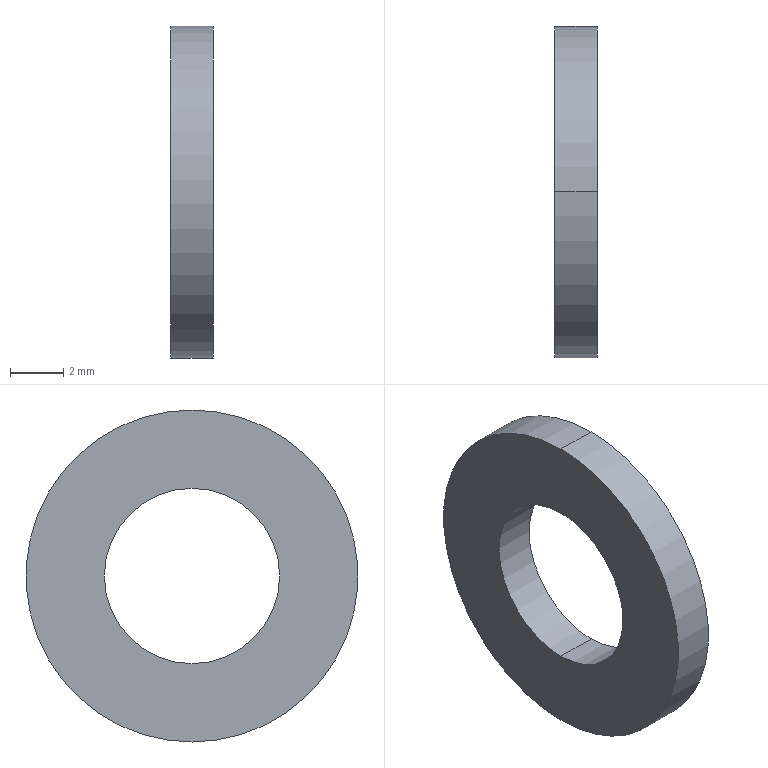Part | STEP file | 0217_303_PFW6 | 1 solid | 6 faces | box 1.6 x 12.5 x 12.5 mm | volume 141.61 mm3 | cylinder 4 | plane 2 | commonest cylinder face diameters 6.6 x2 12.5 x2
STEP:
#1=CARTESIAN_POINT('',(0.,0.,0.));
#2=DIRECTION('',(0.,0.,1.));
#3=DIRECTION('',(1.,0.,0.));
#4=AXIS2_PLACEMENT_3D('',#1,#2,#3);
#5=CARTESIAN_POINT('',(0.,0.,-3.3));
#6=VERTEX_POINT('',#5);
#7=CARTESIAN_POINT('',(1.6,0.,-3.3));
#8=VERTEX_POINT('',#7);
#9=CARTESIAN_POINT('',(0.,0.,-3.3));
#10=DIRECTION('',(1.,0.,0.));
#11=VECTOR('',#10,1.);
#12=LINE('',#9,#11);
#13=CARTESIAN_POINT('',(0.,0.,0.));
#14=DIRECTION('',(1.,0.,0.));
#15=DIRECTION('',(0.,0.,-1.));
#16=AXIS2_PLACEMENT_3D('',#13,#14,#15);
#17=CYLINDRICAL_SURFACE('',#16,3.3);
#18=CARTESIAN_POINT('',(6.283,0.));
#19=DIRECTION('',(0.,1.));
#20=VECTOR('',#19,1.);
#21=LINE('',#18,#20);
#22=(GEOMETRIC_REPRESENTATION_CONTEXT(2)PARAMETRIC_REPRESENTATION_CONTEXT()REPRESENTATION_CONTEXT('',''));
#23=DEFINITIONAL_REPRESENTATION('',(#21),#22);
#24=PCURVE('',#17,#23);
#25=CARTESIAN_POINT('',(0.,0.,0.));
#26=DIRECTION('',(1.,0.,0.));
#27=DIRECTION('',(0.,0.,-1.));
#28=AXIS2_PLACEMENT_3D('',#25,#26,#27);
#29=CYLINDRICAL_SURFACE('',#28,3.3);
#30=CARTESIAN_POINT('',(0.,0.));
#31=DIRECTION('',(0.,1.));
#32=VECTOR('',#31,1.);
#33=LINE('',#30,#32);
#34=(GEOMETRIC_REPRESENTATION_CONTEXT(2)PARAMETRIC_REPRESENTATION_CONTEXT()REPRESENTATION_CONTEXT('',''));
#35=DEFINITIONAL_REPRESENTATION('',(#33),#34);
#36=PCURVE('',#29,#35);
#37=SURFACE_CURVE('',#12,(#24,#36),.PCURVE_S1.);
#38=EDGE_CURVE('',#6,#8,#37,.T.);
#39=ORIENTED_EDGE('',*,*,#38,.T.);
#40=CARTESIAN_POINT('',(1.6,0.,3.3));
#41=VERTEX_POINT('',#40);
#42=CARTESIAN_POINT('',(1.6,0.,0.));
#43=DIRECTION('',(1.,0.,0.));
#44=DIRECTION('',(0.,0.,-1.));
#45=AXIS2_PLACEMENT_3D('',#42,#43,#44);
#46=CIRCLE('',#45,3.3);
#47=CARTESIAN_POINT('',(0.,1.6));
#48=DIRECTION('',(1.,0.));
#49=VECTOR('',#48,1.);
#50=LINE('',#47,#49);
#51=(GEOMETRIC_REPRESENTATION_CONTEXT(2)PARAMETRIC_REPRESENTATION_CONTEXT()REPRESENTATION_CONTEXT('',''));
#52=DEFINITIONAL_REPRESENTATION('',(#50),#51);
#53=PCURVE('',#17,#52);
#54=CARTESIAN_POINT('',(1.6,0.,0.));
#55=DIRECTION('',(-1.,0.,0.));
#56=DIRECTION('',(0.,0.,1.));
#57=AXIS2_PLACEMENT_3D('',#54,#55,#56);
#58=PLANE('',#57);
#59=CARTESIAN_POINT('',(-3.3,0.));
#60=CARTESIAN_POINT('',(-3.3,5.716));
#61=CARTESIAN_POINT('',(1.65,2.858));
#62=CARTESIAN_POINT('',(6.6,0.));
#63=CARTESIAN_POINT('',(1.65,-2.858));
#64=CARTESIAN_POINT('',(-3.3,-5.716));
#65=CARTESIAN_POINT('',(-3.3,0.));
#66=(BOUNDED_CURVE()B_SPLINE_CURVE(2,(#59,#60,#61,#62,#63,#64,#65),.UNSPECIFIED.,.T.,.F.)B_SPLINE_CURVE_WITH_KNOTS((1,2,2,2,2,1),(-2.094,0.,2.094,4.189,6.283,8.378),.UNSPECIFIED.)CURVE()GEOMETRIC_REPRESENTATION_ITEM()RATIONAL_B_SPLINE_CURVE((1.,0.5,1.,0.5,1.,0.5,1.))REPRESENTATION_ITEM(''));
#67=(GEOMETRIC_REPRESENTATION_CONTEXT(2)PARAMETRIC_REPRESENTATION_CONTEXT()REPRESENTATION_CONTEXT('',''));
#68=DEFINITIONAL_REPRESENTATION('',(#66),#67);
#69=PCURVE('',#58,#68);
#70=SURFACE_CURVE('',#46,(#53,#69),.PCURVE_S1.);
#71=EDGE_CURVE('',#41,#8,#70,.T.);
#72=ORIENTED_EDGE('',*,*,#71,.F.);
#73=CARTESIAN_POINT('',(0.,0.,3.3));
#74=VERTEX_POINT('',#73);
#75=CARTESIAN_POINT('',(0.,0.,3.3));
#76=DIRECTION('',(1.,0.,0.));
#77=VECTOR('',#76,1.);
#78=LINE('',#75,#77);
#79=CARTESIAN_POINT('',(3.142,0.));
#80=DIRECTION('',(0.,1.));
#81=VECTOR('',#80,1.);
#82=LINE('',#79,#81);
#83=(GEOMETRIC_REPRESENTATION_CONTEXT(2)PARAMETRIC_REPRESENTATION_CONTEXT()REPRESENTATION_CONTEXT('',''));
#84=DEFINITIONAL_REPRESENTATION('',(#82),#83);
#85=PCURVE('',#17,#84);
#86=CARTESIAN_POINT('',(3.142,0.));
#87=DIRECTION('',(0.,1.));
#88=VECTOR('',#87,1.);
#89=LINE('',#86,#88);
#90=(GEOMETRIC_REPRESENTATION_CONTEXT(2)PARAMETRIC_REPRESENTATION_CONTEXT()REPRESENTATION_CONTEXT('',''));
#91=DEFINITIONAL_REPRESENTATION('',(#89),#90);
#92=PCURVE('',#29,#91);
#93=SURFACE_CURVE('',#78,(#85,#92),.PCURVE_S1.);
#94=EDGE_CURVE('',#74,#41,#93,.T.);
#95=ORIENTED_EDGE('',*,*,#94,.F.);
#96=CARTESIAN_POINT('',(0.,0.,0.));
#97=DIRECTION('',(1.,0.,0.));
#98=DIRECTION('',(0.,0.,-1.));
#99=AXIS2_PLACEMENT_3D('',#96,#97,#98);
#100=CIRCLE('',#99,3.3);
#101=CARTESIAN_POINT('',(0.,0.));
#102=DIRECTION('',(1.,0.));
#103=VECTOR('',#102,1.);
#104=LINE('',#101,#103);
#105=(GEOMETRIC_REPRESENTATION_CONTEXT(2)PARAMETRIC_REPRESENTATION_CONTEXT()REPRESENTATION_CONTEXT('',''));
#106=DEFINITIONAL_REPRESENTATION('',(#104),#105);
#107=PCURVE('',#17,#106);
#108=CARTESIAN_POINT('',(0.,0.,0.));
#109=DIRECTION('',(-1.,0.,0.));
#110=DIRECTION('',(0.,0.,1.));
#111=AXIS2_PLACEMENT_3D('',#108,#109,#110);
#112=PLANE('',#111);
#113=CARTESIAN_POINT('',(-3.3,0.));
#114=CARTESIAN_POINT('',(-3.3,5.716));
#115=CARTESIAN_POINT('',(1.65,2.858));
#116=CARTESIAN_POINT('',(6.6,0.));
#117=CARTESIAN_POINT('',(1.65,-2.858));
#118=CARTESIAN_POINT('',(-3.3,-5.716));
#119=CARTESIAN_POINT('',(-3.3,0.));
#120=(BOUNDED_CURVE()B_SPLINE_CURVE(2,(#113,#114,#115,#116,#117,#118,#119),.UNSPECIFIED.,.T.,.F.)B_SPLINE_CURVE_WITH_KNOTS((1,2,2,2,2,1),(-2.094,0.,2.094,4.189,6.283,8.378),.UNSPECIFIED.)CURVE()GEOMETRIC_REPRESENTATION_ITEM()RATIONAL_B_SPLINE_CURVE((1.,0.5,1.,0.5,1.,0.5,1.))REPRESENTATION_ITEM(''));
#121=(GEOMETRIC_REPRESENTATION_CONTEXT(2)PARAMETRIC_REPRESENTATION_CONTEXT()REPRESENTATION_CONTEXT('',''));
#122=DEFINITIONAL_REPRESENTATION('',(#120),#121);
#123=PCURVE('',#112,#122);
#124=SURFACE_CURVE('',#100,(#107,#123),.PCURVE_S1.);
#125=EDGE_CURVE('',#74,#6,#124,.T.);
#126=ORIENTED_EDGE('',*,*,#125,.T.);
#127=EDGE_LOOP('',(#39,#72,#95,#126));
#128=FACE_BOUND('',#127,.F.);
#129=ADVANCED_FACE('',(#128),#17,.F.);
#130=CARTESIAN_POINT('',(0.,0.,-6.25));
#131=VERTEX_POINT('',#130);
#132=CARTESIAN_POINT('',(0.,0.,6.25));
#133=VERTEX_POINT('',#132);
#134=CARTESIAN_POINT('',(0.,0.,0.));
#135=DIRECTION('',(1.,0.,0.));
#136=DIRECTION('',(0.,0.,-1.));
#137=AXIS2_PLACEMENT_3D('',#134,#135,#136);
#138=CIRCLE('',#137,6.25);
#139=CARTESIAN_POINT('',(0.,0.,0.));
#140=DIRECTION('',(1.,0.,0.));
#141=DIRECTION('',(0.,0.,-1.));
#142=AXIS2_PLACEMENT_3D('',#139,#140,#141);
#143=CYLINDRICAL_SURFACE('',#142,6.25);
#144=CARTESIAN_POINT('',(0.,0.));
#145=DIRECTION('',(1.,0.));
#146=VECTOR('',#145,1.);
#147=LINE('',#144,#146);
#148=(GEOMETRIC_REPRESENTATION_CONTEXT(2)PARAMETRIC_REPRESENTATION_CONTEXT()REPRESENTATION_CONTEXT('',''));
#149=DEFINITIONAL_REPRESENTATION('',(#147),#148);
#150=PCURVE('',#143,#149);
#151=CARTESIAN_POINT('',(-6.25,0.));
#152=CARTESIAN_POINT('',(-6.25,10.825));
#153=CARTESIAN_POINT('',(3.125,5.413));
#154=CARTESIAN_POINT('',(12.5,0.));
#155=CARTESIAN_POINT('',(3.125,-5.413));
#156=CARTESIAN_POINT('',(-6.25,-10.825));
#157=CARTESIAN_POINT('',(-6.25,0.));
#158=(BOUNDED_CURVE()B_SPLINE_CURVE(2,(#151,#152,#153,#154,#155,#156,#157),.UNSPECIFIED.,.T.,.F.)B_SPLINE_CURVE_WITH_KNOTS((1,2,2,2,2,1),(-2.094,0.,2.094,4.189,6.283,8.378),.UNSPECIFIED.)CURVE()GEOMETRIC_REPRESENTATION_ITEM()RATIONAL_B_SPLINE_CURVE((1.,0.5,1.,0.5,1.,0.5,1.))REPRESENTATION_ITEM(''));
#159=(GEOMETRIC_REPRESENTATION_CONTEXT(2)PARAMETRIC_REPRESENTATION_CONTEXT()REPRESENTATION_CONTEXT('',''));
#160=DEFINITIONAL_REPRESENTATION('',(#158),#159);
#161=PCURVE('',#112,#160);
#162=SURFACE_CURVE('',#138,(#150,#161),.PCURVE_S1.);
#163=EDGE_CURVE('',#131,#133,#162,.T.);
#164=ORIENTED_EDGE('',*,*,#163,.T.);
#165=CARTESIAN_POINT('',(1.6,0.,6.25));
#166=VERTEX_POINT('',#165);
#167=CARTESIAN_POINT('',(0.,0.,6.25));
#168=DIRECTION('',(1.,0.,0.));
#169=VECTOR('',#168,1.);
#170=LINE('',#167,#169);
#171=CARTESIAN_POINT('',(3.142,0.));
#172=DIRECTION('',(0.,1.));
#173=VECTOR('',#172,1.);
#174=LINE('',#171,#173);
#175=(GEOMETRIC_REPRESENTATION_CONTEXT(2)PARAMETRIC_REPRESENTATION_CONTEXT()REPRESENTATION_CONTEXT('',''));
#176=DEFINITIONAL_REPRESENTATION('',(#174),#175);
#177=PCURVE('',#143,#176);
#178=CARTESIAN_POINT('',(0.,0.,0.));
#179=DIRECTION('',(1.,0.,0.));
#180=DIRECTION('',(0.,0.,-1.));
#181=AXIS2_PLACEMENT_3D('',#178,#179,#180);
#182=CYLINDRICAL_SURFACE('',#181,6.25);
#183=CARTESIAN_POINT('',(3.142,0.));
#184=DIRECTION('',(0.,1.));
#185=VECTOR('',#184,1.);
#186=LINE('',#183,#185);
#187=(GEOMETRIC_REPRESENTATION_CONTEXT(2)PARAMETRIC_REPRESENTATION_CONTEXT()REPRESENTATION_CONTEXT('',''));
#188=DEFINITIONAL_REPRESENTATION('',(#186),#187);
#189=PCURVE('',#182,#188);
#190=SURFACE_CURVE('',#170,(#177,#189),.PCURVE_S1.);
#191=EDGE_CURVE('',#133,#166,#190,.T.);
#192=ORIENTED_EDGE('',*,*,#191,.T.);
#193=CARTESIAN_POINT('',(1.6,0.,-6.25));
#194=VERTEX_POINT('',#193);
#195=CARTESIAN_POINT('',(1.6,0.,0.));
#196=DIRECTION('',(-1.,0.,0.));
#197=DIRECTION('',(0.,0.,-1.));
#198=AXIS2_PLACEMENT_3D('',#195,#196,#197);
#199=CIRCLE('',#198,6.25);
#200=CARTESIAN_POINT('',(6.283,1.6));
#201=DIRECTION('',(-1.,0.));
#202=VECTOR('',#201,1.);
#203=LINE('',#200,#202);
#204=(GEOMETRIC_REPRESENTATION_CONTEXT(2)PARAMETRIC_REPRESENTATION_CONTEXT()REPRESENTATION_CONTEXT('',''));
#205=DEFINITIONAL_REPRESENTATION('',(#203),#204);
#206=PCURVE('',#143,#205);
#207=CARTESIAN_POINT('',(0.,0.));
#208=DIRECTION('',(-1.,0.));
#209=AXIS2_PLACEMENT_2D('',#207,#208);
#210=CIRCLE('',#209,6.25);
#211=(GEOMETRIC_REPRESENTATION_CONTEXT(2)PARAMETRIC_REPRESENTATION_CONTEXT()REPRESENTATION_CONTEXT('',''));
#212=DEFINITIONAL_REPRESENTATION('',(#210),#211);
#213=PCURVE('',#58,#212);
#214=SURFACE_CURVE('',#199,(#206,#213),.PCURVE_S1.);
#215=EDGE_CURVE('',#166,#194,#214,.T.);
#216=ORIENTED_EDGE('',*,*,#215,.T.);
#217=CARTESIAN_POINT('',(0.,0.,-6.25));
#218=DIRECTION('',(1.,0.,0.));
#219=VECTOR('',#218,1.);
#220=LINE('',#217,#219);
#221=CARTESIAN_POINT('',(0.,0.));
#222=DIRECTION('',(0.,1.));
#223=VECTOR('',#222,1.);
#224=LINE('',#221,#223);
#225=(GEOMETRIC_REPRESENTATION_CONTEXT(2)PARAMETRIC_REPRESENTATION_CONTEXT()REPRESENTATION_CONTEXT('',''));
#226=DEFINITIONAL_REPRESENTATION('',(#224),#225);
#227=PCURVE('',#143,#226);
#228=CARTESIAN_POINT('',(6.283,0.));
#229=DIRECTION('',(0.,1.));
#230=VECTOR('',#229,1.);
#231=LINE('',#228,#230);
#232=(GEOMETRIC_REPRESENTATION_CONTEXT(2)PARAMETRIC_REPRESENTATION_CONTEXT()REPRESENTATION_CONTEXT('',''));
#233=DEFINITIONAL_REPRESENTATION('',(#231),#232);
#234=PCURVE('',#182,#233);
#235=SURFACE_CURVE('',#220,(#227,#234),.PCURVE_S1.);
#236=EDGE_CURVE('',#131,#194,#235,.T.);
#237=ORIENTED_EDGE('',*,*,#236,.F.);
#238=EDGE_LOOP('',(#164,#192,#216,#237));
#239=FACE_BOUND('',#238,.T.);
#240=ADVANCED_FACE('',(#239),#143,.T.);
#241=CARTESIAN_POINT('',(1.6,0.,0.));
#242=DIRECTION('',(1.,0.,0.));
#243=DIRECTION('',(0.,0.,-1.));
#244=AXIS2_PLACEMENT_3D('',#241,#242,#243);
#245=CIRCLE('',#244,3.3);
#246=CARTESIAN_POINT('',(-3.3,0.));
#247=CARTESIAN_POINT('',(-3.3,5.716));
#248=CARTESIAN_POINT('',(1.65,2.858));
#249=CARTESIAN_POINT('',(6.6,0.));
#250=CARTESIAN_POINT('',(1.65,-2.858));
#251=CARTESIAN_POINT('',(-3.3,-5.716));
#252=CARTESIAN_POINT('',(-3.3,0.));
#253=(BOUNDED_CURVE()B_SPLINE_CURVE(2,(#246,#247,#248,#249,#250,#251,#252),.UNSPECIFIED.,.T.,.F.)B_SPLINE_CURVE_WITH_KNOTS((1,2,2,2,2,1),(-2.094,0.,2.094,4.189,6.283,8.378),.UNSPECIFIED.)CURVE()GEOMETRIC_REPRESENTATION_ITEM()RATIONAL_B_SPLINE_CURVE((1.,0.5,1.,0.5,1.,0.5,1.))REPRESENTATION_ITEM(''));
#254=(GEOMETRIC_REPRESENTATION_CONTEXT(2)PARAMETRIC_REPRESENTATION_CONTEXT()REPRESENTATION_CONTEXT('',''));
#255=DEFINITIONAL_REPRESENTATION('',(#253),#254);
#256=PCURVE('',#58,#255);
#257=CARTESIAN_POINT('',(0.,1.6));
#258=DIRECTION('',(1.,0.));
#259=VECTOR('',#258,1.);
#260=LINE('',#257,#259);
#261=(GEOMETRIC_REPRESENTATION_CONTEXT(2)PARAMETRIC_REPRESENTATION_CONTEXT()REPRESENTATION_CONTEXT('',''));
#262=DEFINITIONAL_REPRESENTATION('',(#260),#261);
#263=PCURVE('',#29,#262);
#264=SURFACE_CURVE('',#245,(#256,#263),.PCURVE_S1.);
#265=EDGE_CURVE('',#8,#41,#264,.T.);
#266=ORIENTED_EDGE('',*,*,#265,.F.);
#267=ORIENTED_EDGE('',*,*,#71,.F.);
#268=EDGE_LOOP('',(#266,#267));
#269=FACE_BOUND('',#268,.T.);
#270=CARTESIAN_POINT('',(1.6,0.,0.));
#271=DIRECTION('',(-1.,0.,0.));
#272=DIRECTION('',(0.,0.,-1.));
#273=AXIS2_PLACEMENT_3D('',#270,#271,#272);
#274=CIRCLE('',#273,6.25);
#275=CARTESIAN_POINT('',(0.,0.));
#276=DIRECTION('',(-1.,0.));
#277=AXIS2_PLACEMENT_2D('',#275,#276);
#278=CIRCLE('',#277,6.25);
#279=(GEOMETRIC_REPRESENTATION_CONTEXT(2)PARAMETRIC_REPRESENTATION_CONTEXT()REPRESENTATION_CONTEXT('',''));
#280=DEFINITIONAL_REPRESENTATION('',(#278),#279);
#281=PCURVE('',#58,#280);
#282=CARTESIAN_POINT('',(6.283,1.6));
#283=DIRECTION('',(-1.,0.));
#284=VECTOR('',#283,1.);
#285=LINE('',#282,#284);
#286=(GEOMETRIC_REPRESENTATION_CONTEXT(2)PARAMETRIC_REPRESENTATION_CONTEXT()REPRESENTATION_CONTEXT('',''));
#287=DEFINITIONAL_REPRESENTATION('',(#285),#286);
#288=PCURVE('',#182,#287);
#289=SURFACE_CURVE('',#274,(#281,#288),.PCURVE_S1.);
#290=EDGE_CURVE('',#194,#166,#289,.T.);
#291=ORIENTED_EDGE('',*,*,#290,.F.);
#292=ORIENTED_EDGE('',*,*,#215,.F.);
#293=EDGE_LOOP('',(#291,#292));
#294=FACE_BOUND('',#293,.T.);
#295=ADVANCED_FACE('',(#269,#294),#58,.F.);
#296=ORIENTED_EDGE('',*,*,#265,.F.);
#297=ORIENTED_EDGE('',*,*,#38,.F.);
#298=CARTESIAN_POINT('',(0.,0.,0.));
#299=DIRECTION('',(1.,0.,0.));
#300=DIRECTION('',(0.,0.,-1.));
#301=AXIS2_PLACEMENT_3D('',#298,#299,#300);
#302=CIRCLE('',#301,3.3);
#303=CARTESIAN_POINT('',(0.,0.));
#304=DIRECTION('',(1.,0.));
#305=VECTOR('',#304,1.);
#306=LINE('',#303,#305);
#307=(GEOMETRIC_REPRESENTATION_CONTEXT(2)PARAMETRIC_REPRESENTATION_CONTEXT()REPRESENTATION_CONTEXT('',''));
#308=DEFINITIONAL_REPRESENTATION('',(#306),#307);
#309=PCURVE('',#29,#308);
#310=CARTESIAN_POINT('',(-3.3,0.));
#311=CARTESIAN_POINT('',(-3.3,5.716));
#312=CARTESIAN_POINT('',(1.65,2.858));
#313=CARTESIAN_POINT('',(6.6,0.));
#314=CARTESIAN_POINT('',(1.65,-2.858));
#315=CARTESIAN_POINT('',(-3.3,-5.716));
#316=CARTESIAN_POINT('',(-3.3,0.));
#317=(BOUNDED_CURVE()B_SPLINE_CURVE(2,(#310,#311,#312,#313,#314,#315,#316),.UNSPECIFIED.,.T.,.F.)B_SPLINE_CURVE_WITH_KNOTS((1,2,2,2,2,1),(-2.094,0.,2.094,4.189,6.283,8.378),.UNSPECIFIED.)CURVE()GEOMETRIC_REPRESENTATION_ITEM()RATIONAL_B_SPLINE_CURVE((1.,0.5,1.,0.5,1.,0.5,1.))REPRESENTATION_ITEM(''));
#318=(GEOMETRIC_REPRESENTATION_CONTEXT(2)PARAMETRIC_REPRESENTATION_CONTEXT()REPRESENTATION_CONTEXT('',''));
#319=DEFINITIONAL_REPRESENTATION('',(#317),#318);
#320=PCURVE('',#112,#319);
#321=SURFACE_CURVE('',#302,(#309,#320),.PCURVE_S1.);
#322=EDGE_CURVE('',#6,#74,#321,.T.);
#323=ORIENTED_EDGE('',*,*,#322,.T.);
#324=ORIENTED_EDGE('',*,*,#94,.T.);
#325=EDGE_LOOP('',(#296,#297,#323,#324));
#326=FACE_BOUND('',#325,.F.);
#327=ADVANCED_FACE('',(#326),#29,.F.);
#328=ORIENTED_EDGE('',*,*,#191,.F.);
#329=CARTESIAN_POINT('',(0.,0.,0.));
#330=DIRECTION('',(1.,0.,0.));
#331=DIRECTION('',(0.,0.,-1.));
#332=AXIS2_PLACEMENT_3D('',#329,#330,#331);
#333=CIRCLE('',#332,6.25);
#334=CARTESIAN_POINT('',(0.,0.));
#335=DIRECTION('',(1.,0.));
#336=VECTOR('',#335,1.);
#337=LINE('',#334,#336);
#338=(GEOMETRIC_REPRESENTATION_CONTEXT(2)PARAMETRIC_REPRESENTATION_CONTEXT()REPRESENTATION_CONTEXT('',''));
#339=DEFINITIONAL_REPRESENTATION('',(#337),#338);
#340=PCURVE('',#182,#339);
#341=CARTESIAN_POINT('',(-6.25,0.));
#342=CARTESIAN_POINT('',(-6.25,10.825));
#343=CARTESIAN_POINT('',(3.125,5.413));
#344=CARTESIAN_POINT('',(12.5,0.));
#345=CARTESIAN_POINT('',(3.125,-5.413));
#346=CARTESIAN_POINT('',(-6.25,-10.825));
#347=CARTESIAN_POINT('',(-6.25,0.));
#348=(BOUNDED_CURVE()B_SPLINE_CURVE(2,(#341,#342,#343,#344,#345,#346,#347),.UNSPECIFIED.,.T.,.F.)B_SPLINE_CURVE_WITH_KNOTS((1,2,2,2,2,1),(-2.094,0.,2.094,4.189,6.283,8.378),.UNSPECIFIED.)CURVE()GEOMETRIC_REPRESENTATION_ITEM()RATIONAL_B_SPLINE_CURVE((1.,0.5,1.,0.5,1.,0.5,1.))REPRESENTATION_ITEM(''));
#349=(GEOMETRIC_REPRESENTATION_CONTEXT(2)PARAMETRIC_REPRESENTATION_CONTEXT()REPRESENTATION_CONTEXT('',''));
#350=DEFINITIONAL_REPRESENTATION('',(#348),#349);
#351=PCURVE('',#112,#350);
#352=SURFACE_CURVE('',#333,(#340,#351),.PCURVE_S1.);
#353=EDGE_CURVE('',#133,#131,#352,.T.);
#354=ORIENTED_EDGE('',*,*,#353,.T.);
#355=ORIENTED_EDGE('',*,*,#236,.T.);
#356=ORIENTED_EDGE('',*,*,#290,.T.);
#357=EDGE_LOOP('',(#328,#354,#355,#356));
#358=FACE_BOUND('',#357,.T.);
#359=ADVANCED_FACE('',(#358),#182,.T.);
#360=ORIENTED_EDGE('',*,*,#322,.T.);
#361=ORIENTED_EDGE('',*,*,#125,.T.);
#362=EDGE_LOOP('',(#360,#361));
#363=FACE_BOUND('',#362,.T.);
#364=ORIENTED_EDGE('',*,*,#163,.F.);
#365=ORIENTED_EDGE('',*,*,#353,.F.);
#366=EDGE_LOOP('',(#364,#365));
#367=FACE_BOUND('',#366,.T.);
#368=ADVANCED_FACE('',(#363,#367),#112,.T.);
#369=CLOSED_SHELL('',(#129,#240,#295,#327,#359,#368));
#370=MANIFOLD_SOLID_BREP('',#369);
#371=(LENGTH_UNIT()NAMED_UNIT(*)SI_UNIT(.MILLI.,.METRE.));
#372=UNCERTAINTY_MEASURE_WITH_UNIT(LENGTH_MEASURE(0.0000001),#371,'','');
#373=(NAMED_UNIT(*)PLANE_ANGLE_UNIT()SI_UNIT($,.RADIAN.));
#374=(NAMED_UNIT(*)SI_UNIT($,.STERADIAN.)SOLID_ANGLE_UNIT());
#375=(GEOMETRIC_REPRESENTATION_CONTEXT(3)GLOBAL_UNCERTAINTY_ASSIGNED_CONTEXT((#372))GLOBAL_UNIT_ASSIGNED_CONTEXT((#371,#373,#374))REPRESENTATION_CONTEXT('',''));
#376=ADVANCED_BREP_SHAPE_REPRESENTATION('',(#4,#370),#375);